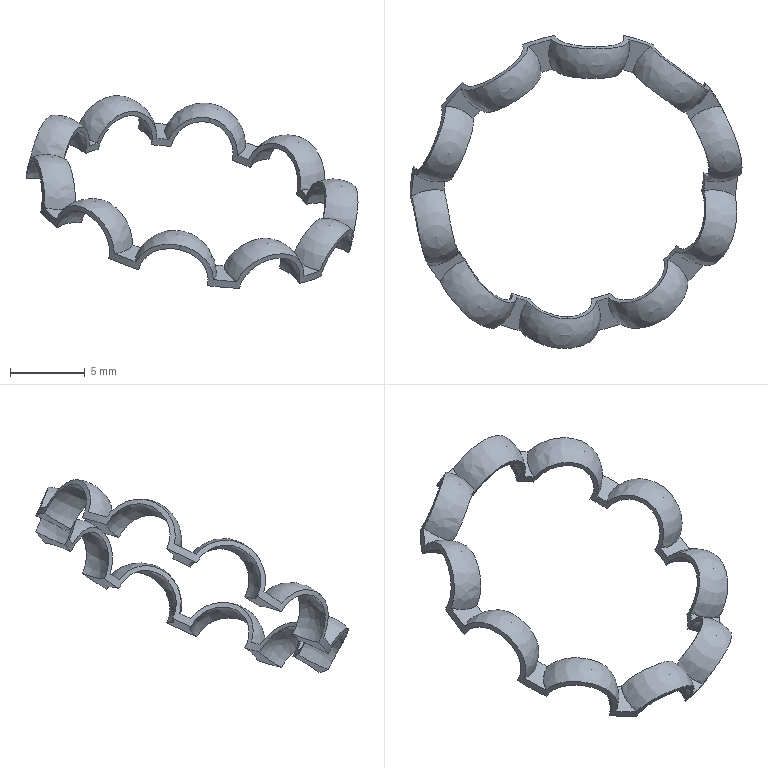Part | SolidWorks | features BaseBody 1 | 1 solid | 44 faces | box 22.149 x 20.875 x 12.86 mm | volume 64.48 mm3 | plane 20 | sphere 18 | cylinder 4 | spline 2 | commonest cylinder face diameters 17.8 x2 22.2 x2